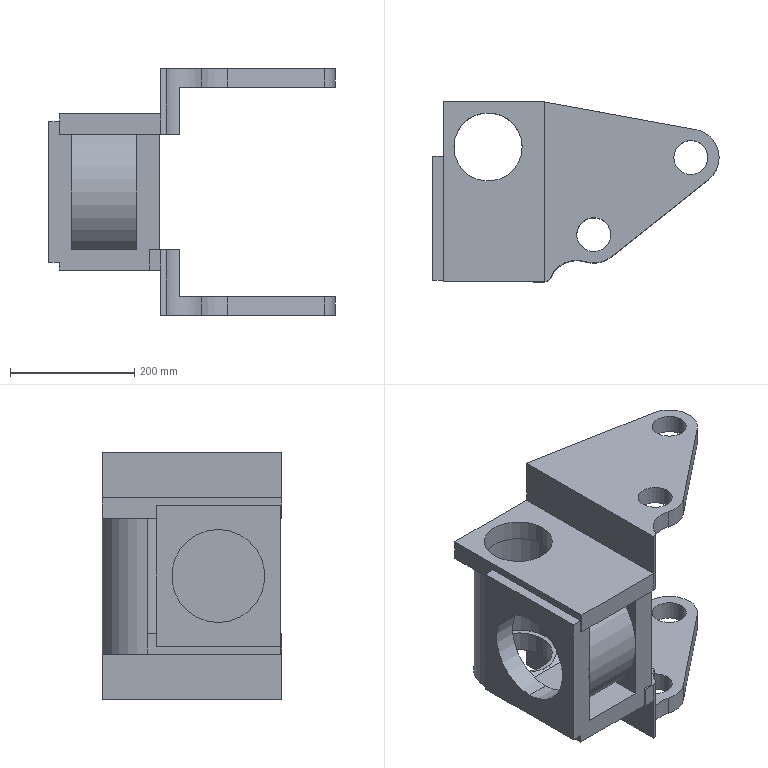Part | SolidWorks | features ICE 16, Extrusion 1, MirrorPattern 1 | 1 solid | 79 faces | box 461.6 x 289.885 x 398 mm | volume 8973124 mm3 | plane 45 | cylinder 34 | commonest cylinder face diameters 55 x8 91.2 x7 110 x4 150 x4 145 x3 198 x3